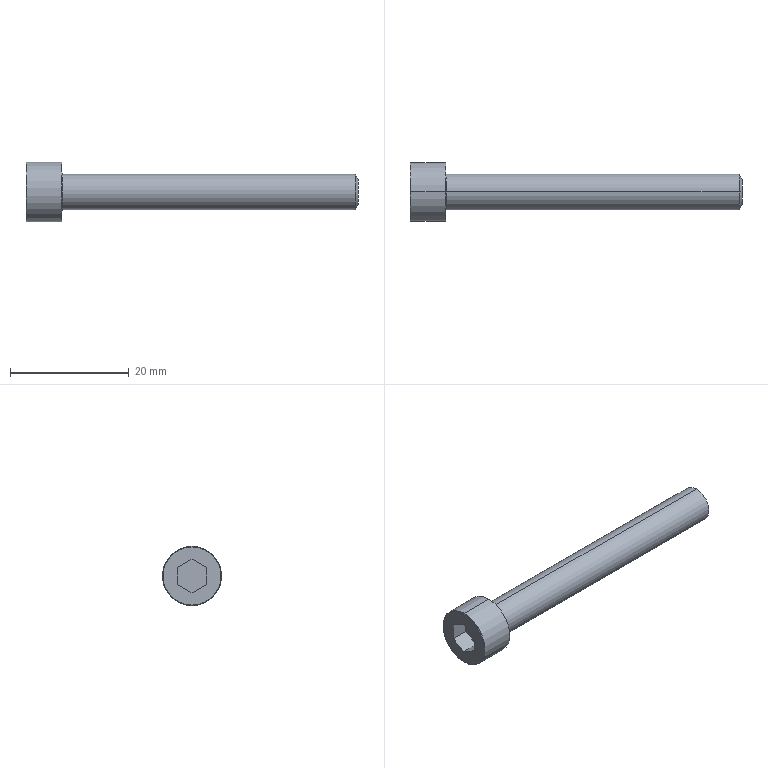Part | SolidWorks | features BlendCut 1, Cut 1, Fillet 1, LPattern 1, RevCut 1, Revolution 1 | 1 solid | 20 faces | box 56 x 10 x 10 mm | volume 1818 mm3 | plane 10 | torus 4 | cylinder 4 | cone 2 | commonest cylinder face diameters 6 x2 10 x2
STEP:
#1=CARTESIAN_POINT('',(0.,0.,4.9));
#2=VERTEX_POINT('',#1);
#3=CARTESIAN_POINT('',(0.,0.,-4.9));
#4=VERTEX_POINT('',#3);
#5=CARTESIAN_POINT('',(0.,0.,0.));
#6=DIRECTION('',(-1.,0.,0.));
#7=DIRECTION('',(0.,0.,-1.));
#8=AXIS2_PLACEMENT_3D('',#5,#6,#7);
#9=CIRCLE('',#8,4.9);
#10=EDGE_CURVE('',#2,#4,#9,.T.);
#11=ORIENTED_EDGE('',*,*,#10,.F.);
#12=CARTESIAN_POINT('',(0.1,0.,5.));
#13=VERTEX_POINT('',#12);
#14=CARTESIAN_POINT('',(0.1,0.,4.9));
#15=DIRECTION('',(0.,1.,0.));
#16=DIRECTION('',(0.,0.,1.));
#17=AXIS2_PLACEMENT_3D('',#14,#15,#16);
#18=CIRCLE('',#17,0.1);
#19=EDGE_CURVE('',#2,#13,#18,.T.);
#20=ORIENTED_EDGE('',*,*,#19,.T.);
#21=CARTESIAN_POINT('',(0.1,0.,-5.));
#22=VERTEX_POINT('',#21);
#23=CARTESIAN_POINT('',(0.1,0.,0.));
#24=DIRECTION('',(1.,0.,0.));
#25=DIRECTION('',(0.,0.,-1.));
#26=AXIS2_PLACEMENT_3D('',#23,#24,#25);
#27=CIRCLE('',#26,5.);
#28=EDGE_CURVE('',#22,#13,#27,.T.);
#29=ORIENTED_EDGE('',*,*,#28,.F.);
#30=CARTESIAN_POINT('',(0.1,0.,-4.9));
#31=DIRECTION('',(0.,-1.,0.));
#32=DIRECTION('',(0.,0.,-1.));
#33=AXIS2_PLACEMENT_3D('',#30,#31,#32);
#34=CIRCLE('',#33,0.1);
#35=EDGE_CURVE('',#4,#22,#34,.T.);
#36=ORIENTED_EDGE('',*,*,#35,.F.);
#37=EDGE_LOOP('',(#11,#20,#29,#36));
#38=FACE_OUTER_BOUND('',#37,.T.);
#39=CARTESIAN_POINT('',(0.1,0.,0.));
#40=DIRECTION('',(1.,0.,0.));
#41=DIRECTION('',(0.,0.,-1.));
#42=AXIS2_PLACEMENT_3D('',#39,#40,#41);
#43=TOROIDAL_SURFACE('',#42,4.9,0.1);
#44=ADVANCED_FACE('',(#38),#43,.T.);
#45=CARTESIAN_POINT('',(56.,0.,2.134));
#46=VERTEX_POINT('',#45);
#47=CARTESIAN_POINT('',(56.,0.,-2.134));
#48=VERTEX_POINT('',#47);
#49=CARTESIAN_POINT('',(56.,0.,0.));
#50=DIRECTION('',(-1.,0.,0.));
#51=DIRECTION('',(0.,0.,1.));
#52=AXIS2_PLACEMENT_3D('',#49,#50,#51);
#53=CIRCLE('',#52,2.134);
#54=EDGE_CURVE('',#46,#48,#53,.T.);
#55=ORIENTED_EDGE('',*,*,#54,.T.);
#56=CARTESIAN_POINT('',(55.5,0.,-3.));
#57=VERTEX_POINT('',#56);
#58=CARTESIAN_POINT('',(55.5,0.,-3.));
#59=DIRECTION('',(-0.5,0.,-0.866));
#60=VECTOR('',#59,1000.);
#61=LINE('',#58,#60);
#62=EDGE_CURVE('',#48,#57,#61,.T.);
#63=ORIENTED_EDGE('',*,*,#62,.T.);
#64=CARTESIAN_POINT('',(55.5,0.,3.));
#65=VERTEX_POINT('',#64);
#66=CARTESIAN_POINT('',(55.5,0.,0.));
#67=DIRECTION('',(-1.,0.,0.));
#68=DIRECTION('',(0.,0.,1.));
#69=AXIS2_PLACEMENT_3D('',#66,#67,#68);
#70=CIRCLE('',#69,3.);
#71=EDGE_CURVE('',#65,#57,#70,.T.);
#72=ORIENTED_EDGE('',*,*,#71,.F.);
#73=CARTESIAN_POINT('',(55.5,0.,3.));
#74=DIRECTION('',(-0.5,0.,0.866));
#75=VECTOR('',#74,1000.);
#76=LINE('',#73,#75);
#77=EDGE_CURVE('',#46,#65,#76,.T.);
#78=ORIENTED_EDGE('',*,*,#77,.F.);
#79=EDGE_LOOP('',(#55,#63,#72,#78));
#80=FACE_OUTER_BOUND('',#79,.T.);
#81=CARTESIAN_POINT('',(55.5,0.,0.));
#82=DIRECTION('',(-1.,0.,0.));
#83=DIRECTION('',(0.,0.,1.));
#84=AXIS2_PLACEMENT_3D('',#81,#82,#83);
#85=CONICAL_SURFACE('',#84,3.,1.047);
#86=ADVANCED_FACE('',(#80),#85,.T.);
#87=CARTESIAN_POINT('',(6.,0.,-3.2));
#88=VERTEX_POINT('',#87);
#89=CARTESIAN_POINT('',(6.,0.,3.2));
#90=VERTEX_POINT('',#89);
#91=CARTESIAN_POINT('',(6.,0.,0.));
#92=DIRECTION('',(-1.,0.,0.));
#93=DIRECTION('',(0.,0.,1.));
#94=AXIS2_PLACEMENT_3D('',#91,#92,#93);
#95=CIRCLE('',#94,3.2);
#96=EDGE_CURVE('',#88,#90,#95,.T.);
#97=ORIENTED_EDGE('',*,*,#96,.F.);
#98=CARTESIAN_POINT('',(6.2,0.,-3.));
#99=VERTEX_POINT('',#98);
#100=CARTESIAN_POINT('',(6.2,0.,-3.2));
#101=DIRECTION('',(0.,1.,0.));
#102=DIRECTION('',(0.,0.,1.));
#103=AXIS2_PLACEMENT_3D('',#100,#101,#102);
#104=CIRCLE('',#103,0.2);
#105=EDGE_CURVE('',#88,#99,#104,.T.);
#106=ORIENTED_EDGE('',*,*,#105,.T.);
#107=CARTESIAN_POINT('',(6.2,0.,3.));
#108=VERTEX_POINT('',#107);
#109=CARTESIAN_POINT('',(6.2,0.,0.));
#110=DIRECTION('',(-1.,0.,0.));
#111=DIRECTION('',(0.,0.,1.));
#112=AXIS2_PLACEMENT_3D('',#109,#110,#111);
#113=CIRCLE('',#112,3.);
#114=EDGE_CURVE('',#99,#108,#113,.T.);
#115=ORIENTED_EDGE('',*,*,#114,.T.);
#116=CARTESIAN_POINT('',(6.2,0.,3.2));
#117=DIRECTION('',(0.,-1.,0.));
#118=DIRECTION('',(0.,0.,-1.));
#119=AXIS2_PLACEMENT_3D('',#116,#117,#118);
#120=CIRCLE('',#119,0.2);
#121=EDGE_CURVE('',#90,#108,#120,.T.);
#122=ORIENTED_EDGE('',*,*,#121,.F.);
#123=EDGE_LOOP('',(#97,#106,#115,#122));
#124=FACE_OUTER_BOUND('',#123,.T.);
#125=CARTESIAN_POINT('',(6.2,0.,0.));
#126=DIRECTION('',(-1.,0.,0.));
#127=DIRECTION('',(0.,0.,1.));
#128=AXIS2_PLACEMENT_3D('',#125,#126,#127);
#129=TOROIDAL_SURFACE('',#128,3.2,0.2);
#130=ADVANCED_FACE('',(#124),#129,.F.);
#131=CARTESIAN_POINT('',(6.,0.,5.));
#132=VERTEX_POINT('',#131);
#133=CARTESIAN_POINT('',(6.,0.,-5.));
#134=VERTEX_POINT('',#133);
#135=CARTESIAN_POINT('',(6.,0.,0.));
#136=DIRECTION('',(-1.,0.,0.));
#137=DIRECTION('',(0.,0.,1.));
#138=AXIS2_PLACEMENT_3D('',#135,#136,#137);
#139=CIRCLE('',#138,5.);
#140=EDGE_CURVE('',#132,#134,#139,.T.);
#141=ORIENTED_EDGE('',*,*,#140,.T.);
#142=CARTESIAN_POINT('',(0.,0.,-5.));
#143=DIRECTION('',(-1.,0.,0.));
#144=VECTOR('',#143,1000.);
#145=LINE('',#142,#144);
#146=EDGE_CURVE('',#134,#22,#145,.T.);
#147=ORIENTED_EDGE('',*,*,#146,.T.);
#148=ORIENTED_EDGE('',*,*,#28,.T.);
#149=CARTESIAN_POINT('',(0.,0.,5.));
#150=DIRECTION('',(-1.,0.,0.));
#151=VECTOR('',#150,1000.);
#152=LINE('',#149,#151);
#153=EDGE_CURVE('',#132,#13,#152,.T.);
#154=ORIENTED_EDGE('',*,*,#153,.F.);
#155=EDGE_LOOP('',(#141,#147,#148,#154));
#156=FACE_OUTER_BOUND('',#155,.T.);
#157=CARTESIAN_POINT('',(0.,0.,0.));
#158=DIRECTION('',(-1.,0.,0.));
#159=DIRECTION('',(0.,0.,1.));
#160=AXIS2_PLACEMENT_3D('',#157,#158,#159);
#161=CYLINDRICAL_SURFACE('',#160,5.);
#162=ADVANCED_FACE('',(#156),#161,.T.);
#163=ORIENTED_EDGE('',*,*,#71,.T.);
#164=CARTESIAN_POINT('',(0.,0.,-3.));
#165=DIRECTION('',(-1.,0.,0.));
#166=VECTOR('',#165,1000.);
#167=LINE('',#164,#166);
#168=EDGE_CURVE('',#57,#99,#167,.T.);
#169=ORIENTED_EDGE('',*,*,#168,.T.);
#170=CARTESIAN_POINT('',(6.2,0.,0.));
#171=DIRECTION('',(-1.,0.,0.));
#172=DIRECTION('',(0.,0.,1.));
#173=AXIS2_PLACEMENT_3D('',#170,#171,#172);
#174=CIRCLE('',#173,3.);
#175=EDGE_CURVE('',#108,#99,#174,.T.);
#176=ORIENTED_EDGE('',*,*,#175,.F.);
#177=CARTESIAN_POINT('',(0.,0.,3.));
#178=DIRECTION('',(-1.,0.,0.));
#179=VECTOR('',#178,1000.);
#180=LINE('',#177,#179);
#181=EDGE_CURVE('',#65,#108,#180,.T.);
#182=ORIENTED_EDGE('',*,*,#181,.F.);
#183=EDGE_LOOP('',(#163,#169,#176,#182));
#184=FACE_OUTER_BOUND('',#183,.T.);
#185=CARTESIAN_POINT('',(0.,0.,0.));
#186=DIRECTION('',(-1.,0.,0.));
#187=DIRECTION('',(0.,0.,1.));
#188=AXIS2_PLACEMENT_3D('',#185,#186,#187);
#189=CYLINDRICAL_SURFACE('',#188,3.);
#190=ADVANCED_FACE('',(#184),#189,.T.);
#191=ORIENTED_EDGE('',*,*,#168,.F.);
#192=CARTESIAN_POINT('',(55.5,0.,0.));
#193=DIRECTION('',(-1.,0.,0.));
#194=DIRECTION('',(0.,0.,1.));
#195=AXIS2_PLACEMENT_3D('',#192,#193,#194);
#196=CIRCLE('',#195,3.);
#197=EDGE_CURVE('',#57,#65,#196,.T.);
#198=ORIENTED_EDGE('',*,*,#197,.T.);
#199=ORIENTED_EDGE('',*,*,#181,.T.);
#200=ORIENTED_EDGE('',*,*,#114,.F.);
#201=EDGE_LOOP('',(#191,#198,#199,#200));
#202=FACE_OUTER_BOUND('',#201,.T.);
#203=CARTESIAN_POINT('',(0.,0.,0.));
#204=DIRECTION('',(-1.,0.,0.));
#205=DIRECTION('',(0.,0.,1.));
#206=AXIS2_PLACEMENT_3D('',#203,#204,#205);
#207=CYLINDRICAL_SURFACE('',#206,3.);
#208=ADVANCED_FACE('',(#202),#207,.T.);
#209=CARTESIAN_POINT('',(0.,0.,0.));
#210=DIRECTION('',(-1.,0.,0.));
#211=DIRECTION('',(0.,0.,-1.));
#212=AXIS2_PLACEMENT_3D('',#209,#210,#211);
#213=CIRCLE('',#212,4.9);
#214=EDGE_CURVE('',#4,#2,#213,.T.);
#215=ORIENTED_EDGE('',*,*,#214,.T.);
#216=ORIENTED_EDGE('',*,*,#10,.T.);
#217=EDGE_LOOP('',(#215,#216));
#218=FACE_OUTER_BOUND('',#217,.T.);
#219=CARTESIAN_POINT('',(0.,0.,2.86));
#220=VERTEX_POINT('',#219);
#221=CARTESIAN_POINT('',(0.,2.477,1.43));
#222=VERTEX_POINT('',#221);
#223=CARTESIAN_POINT('',(0.,0.,2.86));
#224=DIRECTION('',(0.,0.866,-0.5));
#225=VECTOR('',#224,1000.);
#226=LINE('',#223,#225);
#227=EDGE_CURVE('',#220,#222,#226,.T.);
#228=ORIENTED_EDGE('',*,*,#227,.F.);
#229=CARTESIAN_POINT('',(0.,-2.477,1.43));
#230=VERTEX_POINT('',#229);
#231=CARTESIAN_POINT('',(0.,-2.477,1.43));
#232=DIRECTION('',(0.,0.866,0.5));
#233=VECTOR('',#232,1000.);
#234=LINE('',#231,#233);
#235=EDGE_CURVE('',#230,#220,#234,.T.);
#236=ORIENTED_EDGE('',*,*,#235,.F.);
#237=CARTESIAN_POINT('',(0.,-2.477,-1.43));
#238=VERTEX_POINT('',#237);
#239=CARTESIAN_POINT('',(0.,-2.477,-1.43));
#240=DIRECTION('',(0.,0.,1.));
#241=VECTOR('',#240,1000.);
#242=LINE('',#239,#241);
#243=EDGE_CURVE('',#238,#230,#242,.T.);
#244=ORIENTED_EDGE('',*,*,#243,.F.);
#245=CARTESIAN_POINT('',(0.,0.,-2.86));
#246=VERTEX_POINT('',#245);
#247=CARTESIAN_POINT('',(0.,0.,-2.86));
#248=DIRECTION('',(0.,-0.866,0.5));
#249=VECTOR('',#248,1000.);
#250=LINE('',#247,#249);
#251=EDGE_CURVE('',#246,#238,#250,.T.);
#252=ORIENTED_EDGE('',*,*,#251,.F.);
#253=CARTESIAN_POINT('',(0.,2.477,-1.43));
#254=VERTEX_POINT('',#253);
#255=CARTESIAN_POINT('',(0.,2.477,-1.43));
#256=DIRECTION('',(0.,-0.866,-0.5));
#257=VECTOR('',#256,1000.);
#258=LINE('',#255,#257);
#259=EDGE_CURVE('',#254,#246,#258,.T.);
#260=ORIENTED_EDGE('',*,*,#259,.F.);
#261=CARTESIAN_POINT('',(0.,2.477,1.43));
#262=DIRECTION('',(0.,0.,-1.));
#263=VECTOR('',#262,1000.);
#264=LINE('',#261,#263);
#265=EDGE_CURVE('',#222,#254,#264,.T.);
#266=ORIENTED_EDGE('',*,*,#265,.F.);
#267=EDGE_LOOP('',(#228,#236,#244,#252,#260,#266));
#268=FACE_BOUND('',#267,.T.);
#269=CARTESIAN_POINT('',(0.,0.,0.));
#270=DIRECTION('',(1.,0.,0.));
#271=DIRECTION('',(0.,0.,-1.));
#272=AXIS2_PLACEMENT_3D('',#269,#270,#271);
#273=PLANE('',#272);
#274=ADVANCED_FACE('',(#218,#268),#273,.F.);
#275=ORIENTED_EDGE('',*,*,#146,.F.);
#276=CARTESIAN_POINT('',(6.,0.,0.));
#277=DIRECTION('',(-1.,0.,0.));
#278=DIRECTION('',(0.,0.,1.));
#279=AXIS2_PLACEMENT_3D('',#276,#277,#278);
#280=CIRCLE('',#279,5.);
#281=EDGE_CURVE('',#134,#132,#280,.T.);
#282=ORIENTED_EDGE('',*,*,#281,.T.);
#283=ORIENTED_EDGE('',*,*,#153,.T.);
#284=CARTESIAN_POINT('',(0.1,0.,0.));
#285=DIRECTION('',(1.,0.,0.));
#286=DIRECTION('',(0.,0.,-1.));
#287=AXIS2_PLACEMENT_3D('',#284,#285,#286);
#288=CIRCLE('',#287,5.);
#289=EDGE_CURVE('',#13,#22,#288,.T.);
#290=ORIENTED_EDGE('',*,*,#289,.T.);
#291=EDGE_LOOP('',(#275,#282,#283,#290));
#292=FACE_OUTER_BOUND('',#291,.T.);
#293=CARTESIAN_POINT('',(0.,0.,0.));
#294=DIRECTION('',(-1.,0.,0.));
#295=DIRECTION('',(0.,0.,1.));
#296=AXIS2_PLACEMENT_3D('',#293,#294,#295);
#297=CYLINDRICAL_SURFACE('',#296,5.);
#298=ADVANCED_FACE('',(#292),#297,.T.);
#299=ORIENTED_EDGE('',*,*,#140,.F.);
#300=ORIENTED_EDGE('',*,*,#281,.F.);
#301=EDGE_LOOP('',(#299,#300));
#302=FACE_OUTER_BOUND('',#301,.T.);
#303=CARTESIAN_POINT('',(6.,0.,0.));
#304=DIRECTION('',(-1.,0.,0.));
#305=DIRECTION('',(0.,0.,1.));
#306=AXIS2_PLACEMENT_3D('',#303,#304,#305);
#307=CIRCLE('',#306,3.2);
#308=EDGE_CURVE('',#90,#88,#307,.T.);
#309=ORIENTED_EDGE('',*,*,#308,.T.);
#310=ORIENTED_EDGE('',*,*,#96,.T.);
#311=EDGE_LOOP('',(#309,#310));
#312=FACE_BOUND('',#311,.T.);
#313=CARTESIAN_POINT('',(6.,5.,0.));
#314=DIRECTION('',(-1.,0.,0.));
#315=DIRECTION('',(0.,0.,1.));
#316=AXIS2_PLACEMENT_3D('',#313,#314,#315);
#317=PLANE('',#316);
#318=ADVANCED_FACE('',(#302,#312),#317,.F.);
#319=ORIENTED_EDGE('',*,*,#105,.F.);
#320=ORIENTED_EDGE('',*,*,#308,.F.);
#321=ORIENTED_EDGE('',*,*,#121,.T.);
#322=ORIENTED_EDGE('',*,*,#175,.T.);
#323=EDGE_LOOP('',(#319,#320,#321,#322));
#324=FACE_OUTER_BOUND('',#323,.T.);
#325=CARTESIAN_POINT('',(6.2,0.,0.));
#326=DIRECTION('',(-1.,0.,0.));
#327=DIRECTION('',(0.,0.,1.));
#328=AXIS2_PLACEMENT_3D('',#325,#326,#327);
#329=TOROIDAL_SURFACE('',#328,3.2,0.2);
#330=ADVANCED_FACE('',(#324),#329,.F.);
#331=ORIENTED_EDGE('',*,*,#235,.T.);
#332=CARTESIAN_POINT('',(3.,0.,2.86));
#333=VERTEX_POINT('',#332);
#334=CARTESIAN_POINT('',(3.,0.,2.86));
#335=DIRECTION('',(-1.,0.,0.));
#336=VECTOR('',#335,1000.);
#337=LINE('',#334,#336);
#338=EDGE_CURVE('',#333,#220,#337,.T.);
#339=ORIENTED_EDGE('',*,*,#338,.F.);
#340=CARTESIAN_POINT('',(3.,-2.477,1.43));
#341=VERTEX_POINT('',#340);
#342=CARTESIAN_POINT('',(3.,-2.477,1.43));
#343=DIRECTION('',(0.,0.866,0.5));
#344=VECTOR('',#343,1000.);
#345=LINE('',#342,#344);
#346=EDGE_CURVE('',#341,#333,#345,.T.);
#347=ORIENTED_EDGE('',*,*,#346,.F.);
#348=CARTESIAN_POINT('',(3.,-2.477,1.43));
#349=DIRECTION('',(-1.,0.,0.));
#350=VECTOR('',#349,1000.);
#351=LINE('',#348,#350);
#352=EDGE_CURVE('',#341,#230,#351,.T.);
#353=ORIENTED_EDGE('',*,*,#352,.T.);
#354=EDGE_LOOP('',(#331,#339,#347,#353));
#355=FACE_OUTER_BOUND('',#354,.T.);
#356=CARTESIAN_POINT('',(3.,-2.477,1.43));
#357=DIRECTION('',(0.,-0.5,0.866));
#358=DIRECTION('',(0.,-0.866,-0.5));
#359=AXIS2_PLACEMENT_3D('',#356,#357,#358);
#360=PLANE('',#359);
#361=ADVANCED_FACE('',(#355),#360,.F.);
#362=ORIENTED_EDGE('',*,*,#243,.T.);
#363=ORIENTED_EDGE('',*,*,#352,.F.);
#364=CARTESIAN_POINT('',(3.,-2.477,-1.43));
#365=VERTEX_POINT('',#364);
#366=CARTESIAN_POINT('',(3.,-2.477,-1.43));
#367=DIRECTION('',(0.,0.,1.));
#368=VECTOR('',#367,1000.);
#369=LINE('',#366,#368);
#370=EDGE_CURVE('',#365,#341,#369,.T.);
#371=ORIENTED_EDGE('',*,*,#370,.F.);
#372=CARTESIAN_POINT('',(3.,-2.477,-1.43));
#373=DIRECTION('',(-1.,0.,0.));
#374=VECTOR('',#373,1000.);
#375=LINE('',#372,#374);
#376=EDGE_CURVE('',#365,#238,#375,.T.);
#377=ORIENTED_EDGE('',*,*,#376,.T.);
#378=EDGE_LOOP('',(#362,#363,#371,#377));
#379=FACE_OUTER_BOUND('',#378,.T.);
#380=CARTESIAN_POINT('',(3.,-2.477,-1.43));
#381=DIRECTION('',(0.,-1.,0.));
#382=DIRECTION('',(0.,0.,-1.));
#383=AXIS2_PLACEMENT_3D('',#380,#381,#382);
#384=PLANE('',#383);
#385=ADVANCED_FACE('',(#379),#384,.F.);
#386=ORIENTED_EDGE('',*,*,#251,.T.);
#387=ORIENTED_EDGE('',*,*,#376,.F.);
#388=CARTESIAN_POINT('',(3.,0.,-2.86));
#389=VERTEX_POINT('',#388);
#390=CARTESIAN_POINT('',(3.,0.,-2.86));
#391=DIRECTION('',(0.,-0.866,0.5));
#392=VECTOR('',#391,1000.);
#393=LINE('',#390,#392);
#394=EDGE_CURVE('',#389,#365,#393,.T.);
#395=ORIENTED_EDGE('',*,*,#394,.F.);
#396=CARTESIAN_POINT('',(3.,0.,-2.86));
#397=DIRECTION('',(-1.,0.,0.));
#398=VECTOR('',#397,1000.);
#399=LINE('',#396,#398);
#400=EDGE_CURVE('',#389,#246,#399,.T.);
#401=ORIENTED_EDGE('',*,*,#400,.T.);
#402=EDGE_LOOP('',(#386,#387,#395,#401));
#403=FACE_OUTER_BOUND('',#402,.T.);
#404=CARTESIAN_POINT('',(3.,0.,-2.86));
#405=DIRECTION('',(0.,-0.5,-0.866));
#406=DIRECTION('',(0.,0.866,-0.5));
#407=AXIS2_PLACEMENT_3D('',#404,#405,#406);
#408=PLANE('',#407);
#409=ADVANCED_FACE('',(#403),#408,.F.);
#410=ORIENTED_EDGE('',*,*,#259,.T.);
#411=ORIENTED_EDGE('',*,*,#400,.F.);
#412=CARTESIAN_POINT('',(3.,2.477,-1.43));
#413=VERTEX_POINT('',#412);
#414=CARTESIAN_POINT('',(3.,2.477,-1.43));
#415=DIRECTION('',(0.,-0.866,-0.5));
#416=VECTOR('',#415,1000.);
#417=LINE('',#414,#416);
#418=EDGE_CURVE('',#413,#389,#417,.T.);
#419=ORIENTED_EDGE('',*,*,#418,.F.);
#420=CARTESIAN_POINT('',(3.,2.477,-1.43));
#421=DIRECTION('',(-1.,0.,0.));
#422=VECTOR('',#421,1000.);
#423=LINE('',#420,#422);
#424=EDGE_CURVE('',#413,#254,#423,.T.);
#425=ORIENTED_EDGE('',*,*,#424,.T.);
#426=EDGE_LOOP('',(#410,#411,#419,#425));
#427=FACE_OUTER_BOUND('',#426,.T.);
#428=CARTESIAN_POINT('',(3.,2.477,-1.43));
#429=DIRECTION('',(0.,0.5,-0.866));
#430=DIRECTION('',(0.,0.866,0.5));
#431=AXIS2_PLACEMENT_3D('',#428,#429,#430);
#432=PLANE('',#431);
#433=ADVANCED_FACE('',(#427),#432,.F.);
#434=ORIENTED_EDGE('',*,*,#265,.T.);
#435=ORIENTED_EDGE('',*,*,#424,.F.);
#436=CARTESIAN_POINT('',(3.,2.477,1.43));
#437=VERTEX_POINT('',#436);
#438=CARTESIAN_POINT('',(3.,2.477,1.43));
#439=DIRECTION('',(0.,0.,-1.));
#440=VECTOR('',#439,1000.);
#441=LINE('',#438,#440);
#442=EDGE_CURVE('',#437,#413,#441,.T.);
#443=ORIENTED_EDGE('',*,*,#442,.F.);
#444=CARTESIAN_POINT('',(3.,2.477,1.43));
#445=DIRECTION('',(-1.,0.,0.));
#446=VECTOR('',#445,1000.);
#447=LINE('',#444,#446);
#448=EDGE_CURVE('',#437,#222,#447,.T.);
#449=ORIENTED_EDGE('',*,*,#448,.T.);
#450=EDGE_LOOP('',(#434,#435,#443,#449));
#451=FACE_OUTER_BOUND('',#450,.T.);
#452=CARTESIAN_POINT('',(3.,2.477,1.43));
#453=DIRECTION('',(0.,1.,0.));
#454=DIRECTION('',(0.,0.,1.));
#455=AXIS2_PLACEMENT_3D('',#452,#453,#454);
#456=PLANE('',#455);
#457=ADVANCED_FACE('',(#451),#456,.F.);
#458=ORIENTED_EDGE('',*,*,#227,.T.);
#459=ORIENTED_EDGE('',*,*,#448,.F.);
#460=CARTESIAN_POINT('',(3.,0.,2.86));
#461=DIRECTION('',(0.,0.866,-0.5));
#462=VECTOR('',#461,1000.);
#463=LINE('',#460,#462);
#464=EDGE_CURVE('',#333,#437,#463,.T.);
#465=ORIENTED_EDGE('',*,*,#464,.F.);
#466=ORIENTED_EDGE('',*,*,#338,.T.);
#467=EDGE_LOOP('',(#458,#459,#465,#466));
#468=FACE_OUTER_BOUND('',#467,.T.);
#469=CARTESIAN_POINT('',(3.,0.,2.86));
#470=DIRECTION('',(0.,0.5,0.866));
#471=DIRECTION('',(0.,-0.866,0.5));
#472=AXIS2_PLACEMENT_3D('',#469,#470,#471);
#473=PLANE('',#472);
#474=ADVANCED_FACE('',(#468),#473,.F.);
#475=ORIENTED_EDGE('',*,*,#346,.T.);
#476=ORIENTED_EDGE('',*,*,#464,.T.);
#477=ORIENTED_EDGE('',*,*,#442,.T.);
#478=ORIENTED_EDGE('',*,*,#418,.T.);
#479=ORIENTED_EDGE('',*,*,#394,.T.);
#480=ORIENTED_EDGE('',*,*,#370,.T.);
#481=EDGE_LOOP('',(#475,#476,#477,#478,#479,#480));
#482=FACE_OUTER_BOUND('',#481,.T.);
#483=CARTESIAN_POINT('',(3.,-2.477,1.43));
#484=DIRECTION('',(1.,0.,0.));
#485=DIRECTION('',(0.,0.,-1.));
#486=AXIS2_PLACEMENT_3D('',#483,#484,#485);
#487=PLANE('',#486);
#488=ADVANCED_FACE('',(#482),#487,.F.);
#489=ORIENTED_EDGE('',*,*,#62,.F.);
#490=CARTESIAN_POINT('',(56.,0.,0.));
#491=DIRECTION('',(-1.,0.,0.));
#492=DIRECTION('',(0.,0.,1.));
#493=AXIS2_PLACEMENT_3D('',#490,#491,#492);
#494=CIRCLE('',#493,2.134);
#495=EDGE_CURVE('',#48,#46,#494,.T.);
#496=ORIENTED_EDGE('',*,*,#495,.T.);
#497=ORIENTED_EDGE('',*,*,#77,.T.);
#498=ORIENTED_EDGE('',*,*,#197,.F.);
#499=EDGE_LOOP('',(#489,#496,#497,#498));
#500=FACE_OUTER_BOUND('',#499,.T.);
#501=CARTESIAN_POINT('',(55.5,0.,0.));
#502=DIRECTION('',(-1.,0.,0.));
#503=DIRECTION('',(0.,0.,1.));
#504=AXIS2_PLACEMENT_3D('',#501,#502,#503);
#505=CONICAL_SURFACE('',#504,3.,1.047);
#506=ADVANCED_FACE('',(#500),#505,.T.);
#507=ORIENTED_EDGE('',*,*,#54,.F.);
#508=ORIENTED_EDGE('',*,*,#495,.F.);
#509=EDGE_LOOP('',(#507,#508));
#510=FACE_OUTER_BOUND('',#509,.T.);
#511=CARTESIAN_POINT('',(56.,3.,0.));
#512=DIRECTION('',(-1.,0.,0.));
#513=DIRECTION('',(0.,0.,1.));
#514=AXIS2_PLACEMENT_3D('',#511,#512,#513);
#515=PLANE('',#514);
#516=ADVANCED_FACE('',(#510),#515,.F.);
#517=ORIENTED_EDGE('',*,*,#19,.F.);
#518=ORIENTED_EDGE('',*,*,#214,.F.);
#519=ORIENTED_EDGE('',*,*,#35,.T.);
#520=ORIENTED_EDGE('',*,*,#289,.F.);
#521=EDGE_LOOP('',(#517,#518,#519,#520));
#522=FACE_OUTER_BOUND('',#521,.T.);
#523=CARTESIAN_POINT('',(0.1,0.,0.));
#524=DIRECTION('',(1.,0.,0.));
#525=DIRECTION('',(0.,0.,-1.));
#526=AXIS2_PLACEMENT_3D('',#523,#524,#525);
#527=TOROIDAL_SURFACE('',#526,4.9,0.1);
#528=ADVANCED_FACE('',(#522),#527,.T.);
#529=CLOSED_SHELL('',(#44,#86,#130,#162,#190,#208,#274,#298,#318,#330,#361,#385,#409,#433,#457,#474,#488,#506,#516,#528));
#530=MANIFOLD_SOLID_BREP('',#529);
#531=CARTESIAN_POINT('',(0.,0.,0.));
#532=DIRECTION('',(0.,0.,1.));
#533=DIRECTION('',(1.,0.,0.));
#534=AXIS2_PLACEMENT_3D('',#531,#532,#533);
#535=(LENGTH_UNIT()NAMED_UNIT(*)SI_UNIT(.MILLI.,.METRE.));
#536=UNCERTAINTY_MEASURE_WITH_UNIT(LENGTH_MEASURE(0.00001),#535,'','');
#537=(NAMED_UNIT(*)PLANE_ANGLE_UNIT()SI_UNIT($,.RADIAN.));
#538=(NAMED_UNIT(*)SI_UNIT($,.STERADIAN.)SOLID_ANGLE_UNIT());
#539=(GEOMETRIC_REPRESENTATION_CONTEXT(3)GLOBAL_UNCERTAINTY_ASSIGNED_CONTEXT((#536))GLOBAL_UNIT_ASSIGNED_CONTEXT((#535,#537,#538))REPRESENTATION_CONTEXT('',''));
#540=ADVANCED_BREP_SHAPE_REPRESENTATION('',(#530,#534),#539);